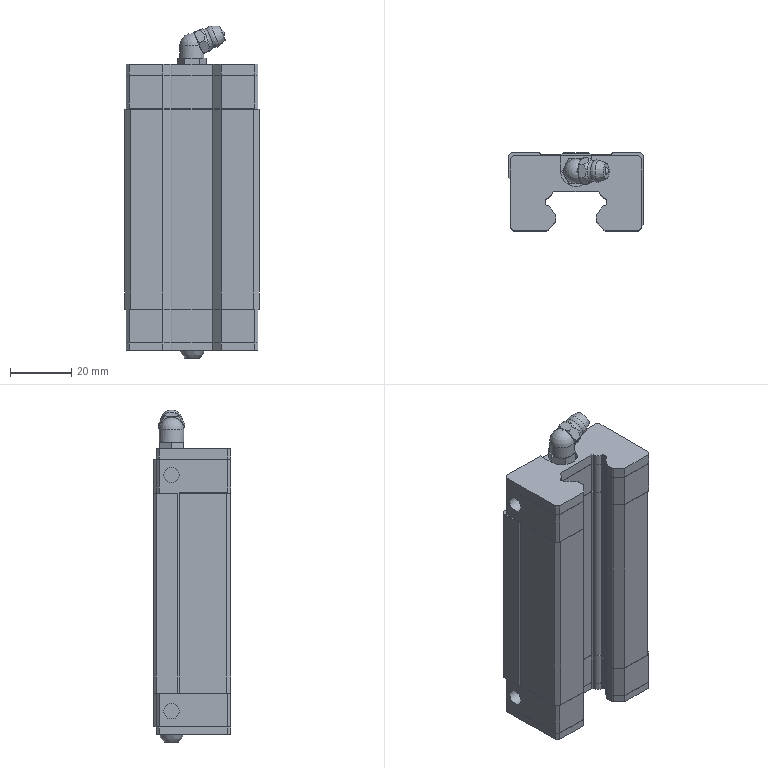Part | STEP file | C-HLGHAB20 | 1 solid | 526 faces | box 44 x 25.4 x 108.25 mm | volume 81548 mm3 | plane 310 | cylinder 204 | cone 6 | spline 2 | sphere 2 | torus 2 | commonest cylinder face diameters 1 x64 1.1 x48 2 x24 4.06 x20 1.9 x16 3.96 x16